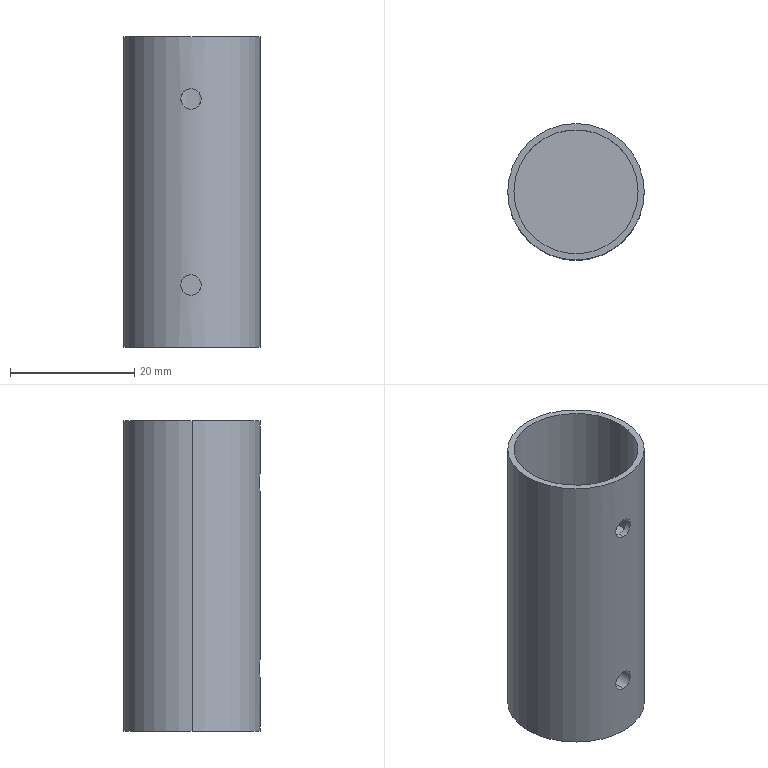Part | NX | 1 solid | 18 faces | box 22 x 22 x 50 mm | volume 7499 mm3 | plane 10 | cylinder 8 | commonest cylinder face diameters 3.3 x4 20 x2 22 x2
STEP:
#1=CARTESIAN_POINT('',(-0.1668,-10.999,38.35));
#2=VERTEX_POINT('',#1);
#3=CARTESIAN_POINT('',(-0.1668,-10.999,41.65));
#4=VERTEX_POINT('',#3);
#5=CARTESIAN_POINT('',(-0.1668,-10.999,38.35));
#6=CARTESIAN_POINT('',(-0.3506,-10.996,38.35));
#7=CARTESIAN_POINT('',(-0.5369,-10.988,38.382));
#8=CARTESIAN_POINT('',(-0.7102,-10.977,38.442));
#9=CARTESIAN_POINT('',(-0.8833,-10.966,38.502));
#10=CARTESIAN_POINT('',(-1.048,-10.951,38.593));
#11=CARTESIAN_POINT('',(-1.192,-10.935,38.707));
#12=CARTESIAN_POINT('',(-1.336,-10.919,38.822));
#13=CARTESIAN_POINT('',(-1.463,-10.903,38.963));
#14=CARTESIAN_POINT('',(-1.562,-10.889,39.119));
#15=CARTESIAN_POINT('',(-1.661,-10.874,39.275));
#16=CARTESIAN_POINT('',(-1.734,-10.863,39.452));
#17=CARTESIAN_POINT('',(-1.775,-10.856,39.633));
#18=CARTESIAN_POINT('',(-1.816,-10.849,39.812));
#19=CARTESIAN_POINT('',(-1.827,-10.847,40.001));
#20=CARTESIAN_POINT('',(-1.807,-10.851,40.184));
#21=CARTESIAN_POINT('',(-1.786,-10.854,40.365));
#22=CARTESIAN_POINT('',(-1.735,-10.863,40.545));
#23=CARTESIAN_POINT('',(-1.656,-10.875,40.71));
#24=CARTESIAN_POINT('',(-1.578,-10.887,40.875));
#25=CARTESIAN_POINT('',(-1.47,-10.902,41.028));
#26=CARTESIAN_POINT('',(-1.342,-10.918,41.158));
#27=CARTESIAN_POINT('',(-1.212,-10.934,41.29));
#28=CARTESIAN_POINT('',(-1.058,-10.95,41.401));
#29=CARTESIAN_POINT('',(-0.8922,-10.964,41.482));
#30=CARTESIAN_POINT('',(-0.7258,-10.977,41.563));
#31=CARTESIAN_POINT('',(-0.5427,-10.988,41.617));
#32=CARTESIAN_POINT('',(-0.3582,-10.994,41.639));
#33=CARTESIAN_POINT('',(-0.2948,-10.996,41.646));
#34=CARTESIAN_POINT('',(-0.2308,-10.998,41.65));
#35=CARTESIAN_POINT('',(-0.1668,-10.999,41.65));
#36=B_SPLINE_CURVE_WITH_KNOTS('',3,(#5,#6,#7,#8,#9,#10,#11,#12,#13,#14,#15,#16,#17,#18,#19,#20,#21,#22,#23,#24,#25,#26,#27,#28,#29,#30,#31,#32,#33,#34,#35),.UNSPECIFIED.,.F.,.F.,(4,3,3,3,3,3,3,3,3,3,4),(0.,0.1067,0.2134,0.3209,0.4288,0.5357,0.6415,0.7478,0.8555,0.9634,1.),.UNSPECIFIED.);
#37=EDGE_CURVE('',#2,#4,#36,.T.);
#38=ORIENTED_EDGE('',*,*,#37,.F.);
#39=CARTESIAN_POINT('',(-0.1668,-9.999,38.35));
#40=VERTEX_POINT('',#39);
#41=CARTESIAN_POINT('',(-0.1668,-8.66,38.35));
#42=DIRECTION('',(0.,1.,0.));
#43=VECTOR('',#42,1.);
#44=LINE('',#41,#43);
#45=EDGE_CURVE('',#2,#40,#44,.T.);
#46=ORIENTED_EDGE('',*,*,#45,.T.);
#47=CARTESIAN_POINT('',(-0.1668,-9.999,41.65));
#48=VERTEX_POINT('',#47);
#49=CARTESIAN_POINT('',(-0.1668,-9.999,41.65));
#50=CARTESIAN_POINT('',(-0.3505,-9.996,41.65));
#51=CARTESIAN_POINT('',(-0.5365,-9.987,41.618));
#52=CARTESIAN_POINT('',(-0.7096,-9.975,41.558));
#53=CARTESIAN_POINT('',(-0.8825,-9.962,41.498));
#54=CARTESIAN_POINT('',(-1.047,-9.946,41.407));
#55=CARTESIAN_POINT('',(-1.191,-9.929,41.294));
#56=CARTESIAN_POINT('',(-1.335,-9.912,41.18));
#57=CARTESIAN_POINT('',(-1.462,-9.893,41.039));
#58=CARTESIAN_POINT('',(-1.561,-9.877,40.883));
#59=CARTESIAN_POINT('',(-1.66,-9.862,40.726));
#60=CARTESIAN_POINT('',(-1.734,-9.849,40.55));
#61=CARTESIAN_POINT('',(-1.775,-9.841,40.368));
#62=CARTESIAN_POINT('',(-1.816,-9.834,40.189));
#63=CARTESIAN_POINT('',(-1.827,-9.832,40.));
#64=CARTESIAN_POINT('',(-1.807,-9.835,39.817));
#65=CARTESIAN_POINT('',(-1.787,-9.839,39.637));
#66=CARTESIAN_POINT('',(-1.735,-9.849,39.457));
#67=CARTESIAN_POINT('',(-1.658,-9.862,39.293));
#68=CARTESIAN_POINT('',(-1.58,-9.875,39.128));
#69=CARTESIAN_POINT('',(-1.473,-9.892,38.975));
#70=CARTESIAN_POINT('',(-1.345,-9.909,38.845));
#71=CARTESIAN_POINT('',(-1.216,-9.927,38.713));
#72=CARTESIAN_POINT('',(-1.062,-9.945,38.602));
#73=CARTESIAN_POINT('',(-0.8961,-9.96,38.52));
#74=CARTESIAN_POINT('',(-0.7298,-9.975,38.438));
#75=CARTESIAN_POINT('',(-0.5466,-9.987,38.384));
#76=CARTESIAN_POINT('',(-0.362,-9.993,38.362));
#77=CARTESIAN_POINT('',(-0.2973,-9.996,38.354));
#78=CARTESIAN_POINT('',(-0.232,-9.998,38.35));
#79=CARTESIAN_POINT('',(-0.1668,-9.999,38.35));
#80=B_SPLINE_CURVE_WITH_KNOTS('',3,(#49,#50,#51,#52,#53,#54,#55,#56,#57,#58,#59,#60,#61,#62,#63,#64,#65,#66,#67,#68,#69,#70,#71,#72,#73,#74,#75,#76,#77,#78,#79),.UNSPECIFIED.,.F.,.F.,(4,3,3,3,3,3,3,3,3,3,4),(0.,0.1066,0.2131,0.3206,0.4287,0.5354,0.6409,0.747,0.8546,0.9626,1.),.UNSPECIFIED.);
#81=EDGE_CURVE('',#48,#40,#80,.T.);
#82=ORIENTED_EDGE('',*,*,#81,.F.);
#83=CARTESIAN_POINT('',(-0.1668,-8.66,41.65));
#84=DIRECTION('',(0.,1.,0.));
#85=VECTOR('',#84,1.);
#86=LINE('',#83,#85);
#87=EDGE_CURVE('',#4,#48,#86,.T.);
#88=ORIENTED_EDGE('',*,*,#87,.F.);
#89=EDGE_LOOP('',(#38,#46,#82,#88));
#90=FACE_OUTER_BOUND('',#89,.T.);
#91=CARTESIAN_POINT('',(-0.1668,-8.66,40.));
#92=DIRECTION('',(0.,1.,0.));
#93=DIRECTION('',(0.,0.,1.));
#94=AXIS2_PLACEMENT_3D('',#91,#92,#93);
#95=CYLINDRICAL_SURFACE('',#94,1.65);
#96=ADVANCED_FACE('',(#90),#95,.F.);
#97=CARTESIAN_POINT('',(-0.1668,-10.999,8.35));
#98=VERTEX_POINT('',#97);
#99=CARTESIAN_POINT('',(-0.1668,-10.999,11.65));
#100=VERTEX_POINT('',#99);
#101=CARTESIAN_POINT('',(-0.1668,-10.999,8.35));
#102=CARTESIAN_POINT('',(-0.3506,-10.996,8.35));
#103=CARTESIAN_POINT('',(-0.5369,-10.988,8.382));
#104=CARTESIAN_POINT('',(-0.7102,-10.977,8.442));
#105=CARTESIAN_POINT('',(-0.8833,-10.966,8.502));
#106=CARTESIAN_POINT('',(-1.048,-10.951,8.593));
#107=CARTESIAN_POINT('',(-1.192,-10.935,8.707));
#108=CARTESIAN_POINT('',(-1.336,-10.919,8.822));
#109=CARTESIAN_POINT('',(-1.463,-10.903,8.963));
#110=CARTESIAN_POINT('',(-1.562,-10.889,9.119));
#111=CARTESIAN_POINT('',(-1.661,-10.874,9.275));
#112=CARTESIAN_POINT('',(-1.734,-10.863,9.452));
#113=CARTESIAN_POINT('',(-1.775,-10.856,9.633));
#114=CARTESIAN_POINT('',(-1.816,-10.849,9.812));
#115=CARTESIAN_POINT('',(-1.827,-10.847,10.001));
#116=CARTESIAN_POINT('',(-1.807,-10.851,10.184));
#117=CARTESIAN_POINT('',(-1.786,-10.854,10.365));
#118=CARTESIAN_POINT('',(-1.735,-10.863,10.545));
#119=CARTESIAN_POINT('',(-1.656,-10.875,10.71));
#120=CARTESIAN_POINT('',(-1.578,-10.887,10.875));
#121=CARTESIAN_POINT('',(-1.47,-10.902,11.028));
#122=CARTESIAN_POINT('',(-1.342,-10.918,11.158));
#123=CARTESIAN_POINT('',(-1.212,-10.934,11.29));
#124=CARTESIAN_POINT('',(-1.058,-10.95,11.401));
#125=CARTESIAN_POINT('',(-0.8922,-10.964,11.482));
#126=CARTESIAN_POINT('',(-0.7258,-10.977,11.563));
#127=CARTESIAN_POINT('',(-0.5427,-10.988,11.617));
#128=CARTESIAN_POINT('',(-0.3582,-10.994,11.639));
#129=CARTESIAN_POINT('',(-0.2948,-10.996,11.646));
#130=CARTESIAN_POINT('',(-0.2308,-10.998,11.65));
#131=CARTESIAN_POINT('',(-0.1668,-10.999,11.65));
#132=B_SPLINE_CURVE_WITH_KNOTS('',3,(#101,#102,#103,#104,#105,#106,#107,#108,#109,#110,#111,#112,#113,#114,#115,#116,#117,#118,#119,#120,#121,#122,#123,#124,#125,#126,#127,#128,#129,#130,#131),.UNSPECIFIED.,.F.,.F.,(4,3,3,3,3,3,3,3,3,3,4),(0.,0.1067,0.2134,0.3209,0.4288,0.5357,0.6415,0.7478,0.8555,0.9634,1.),.UNSPECIFIED.);
#133=EDGE_CURVE('',#98,#100,#132,.T.);
#134=ORIENTED_EDGE('',*,*,#133,.F.);
#135=CARTESIAN_POINT('',(-0.1668,-8.66,8.35));
#136=VERTEX_POINT('',#135);
#137=CARTESIAN_POINT('',(-0.1668,-8.66,8.35));
#138=DIRECTION('',(0.,1.,0.));
#139=VECTOR('',#138,1.);
#140=LINE('',#137,#139);
#141=EDGE_CURVE('',#98,#136,#140,.T.);
#142=ORIENTED_EDGE('',*,*,#141,.T.);
#143=CARTESIAN_POINT('',(-0.1668,-8.66,11.65));
#144=VERTEX_POINT('',#143);
#145=CARTESIAN_POINT('',(-0.1668,-8.66,10.));
#146=DIRECTION('',(0.,1.,0.));
#147=DIRECTION('',(0.,0.,1.));
#148=AXIS2_PLACEMENT_3D('',#145,#146,#147);
#149=CIRCLE('',#148,1.65);
#150=EDGE_CURVE('',#136,#144,#149,.T.);
#151=ORIENTED_EDGE('',*,*,#150,.T.);
#152=CARTESIAN_POINT('',(-0.1668,-8.66,11.65));
#153=DIRECTION('',(0.,1.,0.));
#154=VECTOR('',#153,1.);
#155=LINE('',#152,#154);
#156=EDGE_CURVE('',#100,#144,#155,.T.);
#157=ORIENTED_EDGE('',*,*,#156,.F.);
#158=EDGE_LOOP('',(#134,#142,#151,#157));
#159=FACE_OUTER_BOUND('',#158,.T.);
#160=CARTESIAN_POINT('',(-0.1668,-8.66,10.));
#161=DIRECTION('',(0.,1.,0.));
#162=DIRECTION('',(0.,0.,1.));
#163=AXIS2_PLACEMENT_3D('',#160,#161,#162);
#164=CYLINDRICAL_SURFACE('',#163,1.65);
#165=ADVANCED_FACE('',(#159),#164,.F.);
#166=ORIENTED_EDGE('',*,*,#81,.T.);
#167=CARTESIAN_POINT('',(-0.1668,-9.999,38.35));
#168=CARTESIAN_POINT('',(0.01615,-10.002,38.35));
#169=CARTESIAN_POINT('',(0.2018,-9.999,38.381));
#170=CARTESIAN_POINT('',(0.3745,-9.993,38.441));
#171=CARTESIAN_POINT('',(0.5473,-9.987,38.501));
#172=CARTESIAN_POINT('',(0.7119,-9.976,38.592));
#173=CARTESIAN_POINT('',(0.8552,-9.963,38.705));
#174=CARTESIAN_POINT('',(0.9996,-9.951,38.819));
#175=CARTESIAN_POINT('',(1.126,-9.937,38.959));
#176=CARTESIAN_POINT('',(1.225,-9.925,39.114));
#177=CARTESIAN_POINT('',(1.324,-9.912,39.27));
#178=CARTESIAN_POINT('',(1.398,-9.902,39.446));
#179=CARTESIAN_POINT('',(1.44,-9.896,39.626));
#180=CARTESIAN_POINT('',(1.482,-9.89,39.806));
#181=CARTESIAN_POINT('',(1.493,-9.888,39.995));
#182=CARTESIAN_POINT('',(1.473,-9.891,40.178));
#183=CARTESIAN_POINT('',(1.454,-9.894,40.36));
#184=CARTESIAN_POINT('',(1.403,-9.901,40.541));
#185=CARTESIAN_POINT('',(1.325,-9.912,40.706));
#186=CARTESIAN_POINT('',(1.246,-9.922,40.871));
#187=CARTESIAN_POINT('',(1.139,-9.936,41.026));
#188=CARTESIAN_POINT('',(1.01,-9.949,41.156));
#189=CARTESIAN_POINT('',(0.8808,-9.962,41.288));
#190=CARTESIAN_POINT('',(0.7267,-9.975,41.399));
#191=CARTESIAN_POINT('',(0.5606,-9.984,41.481));
#192=CARTESIAN_POINT('',(0.3946,-9.994,41.563));
#193=CARTESIAN_POINT('',(0.2121,-9.999,41.617));
#194=CARTESIAN_POINT('',(0.0283,-10.,41.638));
#195=CARTESIAN_POINT('',(-0.03641,-10.,41.646));
#196=CARTESIAN_POINT('',(-0.1017,-10.,41.65));
#197=CARTESIAN_POINT('',(-0.1668,-9.999,41.65));
#198=B_SPLINE_CURVE_WITH_KNOTS('',3,(#167,#168,#169,#170,#171,#172,#173,#174,#175,#176,#177,#178,#179,#180,#181,#182,#183,#184,#185,#186,#187,#188,#189,#190,#191,#192,#193,#194,#195,#196,#197),.UNSPECIFIED.,.F.,.F.,(4,3,3,3,3,3,3,3,3,3,4),(0.,0.1063,0.2126,0.3197,0.4275,0.5346,0.6408,0.7474,0.855,0.9626,1.),.UNSPECIFIED.);
#199=EDGE_CURVE('',#40,#48,#198,.T.);
#200=ORIENTED_EDGE('',*,*,#199,.T.);
#201=EDGE_LOOP('',(#166,#200));
#202=FACE_BOUND('',#201,.T.);
#203=CARTESIAN_POINT('',(-10.,0.,30.));
#204=VERTEX_POINT('',#203);
#205=CARTESIAN_POINT('',(10.,0.,30.));
#206=VERTEX_POINT('',#205);
#207=CARTESIAN_POINT('',(0.,0.,30.));
#208=DIRECTION('',(0.,0.,1.));
#209=DIRECTION('',(1.,0.,0.));
#210=AXIS2_PLACEMENT_3D('',#207,#208,#209);
#211=CIRCLE('',#210,10.);
#212=EDGE_CURVE('',#204,#206,#211,.T.);
#213=ORIENTED_EDGE('',*,*,#212,.F.);
#214=CARTESIAN_POINT('',(-10.,0.,50.));
#215=VERTEX_POINT('',#214);
#216=CARTESIAN_POINT('',(-10.,0.,30.));
#217=DIRECTION('',(0.,0.,1.));
#218=VECTOR('',#217,1.);
#219=LINE('',#216,#218);
#220=EDGE_CURVE('',#204,#215,#219,.T.);
#221=ORIENTED_EDGE('',*,*,#220,.T.);
#222=CARTESIAN_POINT('',(10.,0.,50.));
#223=VERTEX_POINT('',#222);
#224=CARTESIAN_POINT('',(0.,0.,50.));
#225=DIRECTION('',(0.,0.,1.));
#226=DIRECTION('',(1.,0.,0.));
#227=AXIS2_PLACEMENT_3D('',#224,#225,#226);
#228=CIRCLE('',#227,10.);
#229=EDGE_CURVE('',#215,#223,#228,.T.);
#230=ORIENTED_EDGE('',*,*,#229,.T.);
#231=CARTESIAN_POINT('',(10.,0.,30.));
#232=DIRECTION('',(0.,0.,1.));
#233=VECTOR('',#232,1.);
#234=LINE('',#231,#233);
#235=EDGE_CURVE('',#206,#223,#234,.T.);
#236=ORIENTED_EDGE('',*,*,#235,.F.);
#237=EDGE_LOOP('',(#213,#221,#230,#236));
#238=FACE_BOUND('',#237,.T.);
#239=CARTESIAN_POINT('',(0.,0.,30.));
#240=DIRECTION('',(0.,0.,1.));
#241=DIRECTION('',(1.,0.,0.));
#242=AXIS2_PLACEMENT_3D('',#239,#240,#241);
#243=CYLINDRICAL_SURFACE('',#242,10.);
#244=ADVANCED_FACE('',(#202,#238),#243,.F.);
#245=CARTESIAN_POINT('',(11.,0.,50.));
#246=VERTEX_POINT('',#245);
#247=CARTESIAN_POINT('',(-11.,0.,50.));
#248=VERTEX_POINT('',#247);
#249=CARTESIAN_POINT('',(0.,0.,50.));
#250=DIRECTION('',(0.,0.,1.));
#251=DIRECTION('',(1.,0.,0.));
#252=AXIS2_PLACEMENT_3D('',#249,#250,#251);
#253=CIRCLE('',#252,11.);
#254=EDGE_CURVE('',#246,#248,#253,.T.);
#255=ORIENTED_EDGE('',*,*,#254,.F.);
#256=CARTESIAN_POINT('',(11.,0.,0.));
#257=VERTEX_POINT('',#256);
#258=CARTESIAN_POINT('',(11.,0.,50.));
#259=DIRECTION('',(0.,0.,1.));
#260=VECTOR('',#259,1.);
#261=LINE('',#258,#260);
#262=EDGE_CURVE('',#257,#246,#261,.T.);
#263=ORIENTED_EDGE('',*,*,#262,.F.);
#264=CARTESIAN_POINT('',(-11.,0.,0.));
#265=VERTEX_POINT('',#264);
#266=CARTESIAN_POINT('',(0.,0.,0.));
#267=DIRECTION('',(0.,0.,1.));
#268=DIRECTION('',(1.,0.,0.));
#269=AXIS2_PLACEMENT_3D('',#266,#267,#268);
#270=CIRCLE('',#269,11.);
#271=EDGE_CURVE('',#257,#265,#270,.T.);
#272=ORIENTED_EDGE('',*,*,#271,.T.);
#273=CARTESIAN_POINT('',(-11.,0.,50.));
#274=DIRECTION('',(0.,0.,1.));
#275=VECTOR('',#274,1.);
#276=LINE('',#273,#275);
#277=EDGE_CURVE('',#265,#248,#276,.T.);
#278=ORIENTED_EDGE('',*,*,#277,.T.);
#279=EDGE_LOOP('',(#255,#263,#272,#278));
#280=FACE_OUTER_BOUND('',#279,.T.);
#281=CARTESIAN_POINT('',(0.,0.,50.));
#282=DIRECTION('',(0.,0.,-1.));
#283=DIRECTION('',(-1.,0.,0.));
#284=AXIS2_PLACEMENT_3D('',#281,#282,#283);
#285=CYLINDRICAL_SURFACE('',#284,11.);
#286=ADVANCED_FACE('',(#280),#285,.T.);
#287=ORIENTED_EDGE('',*,*,#262,.T.);
#288=CARTESIAN_POINT('',(0.,0.,50.));
#289=DIRECTION('',(0.,0.,1.));
#290=DIRECTION('',(1.,0.,0.));
#291=AXIS2_PLACEMENT_3D('',#288,#289,#290);
#292=CIRCLE('',#291,11.);
#293=EDGE_CURVE('',#248,#246,#292,.T.);
#294=ORIENTED_EDGE('',*,*,#293,.F.);
#295=ORIENTED_EDGE('',*,*,#277,.F.);
#296=CARTESIAN_POINT('',(0.,0.,0.));
#297=DIRECTION('',(0.,0.,1.));
#298=DIRECTION('',(1.,0.,0.));
#299=AXIS2_PLACEMENT_3D('',#296,#297,#298);
#300=CIRCLE('',#299,11.);
#301=EDGE_CURVE('',#265,#257,#300,.T.);
#302=ORIENTED_EDGE('',*,*,#301,.T.);
#303=EDGE_LOOP('',(#287,#294,#295,#302));
#304=FACE_BOUND('',#303,.T.);
#305=CARTESIAN_POINT('',(-0.1668,-10.999,41.65));
#306=CARTESIAN_POINT('',(0.01644,-11.002,41.65));
#307=CARTESIAN_POINT('',(0.2023,-11.,41.619));
#308=CARTESIAN_POINT('',(0.3754,-10.994,41.558));
#309=CARTESIAN_POINT('',(0.5484,-10.988,41.498));
#310=CARTESIAN_POINT('',(0.7133,-10.978,41.408));
#311=CARTESIAN_POINT('',(0.8567,-10.967,41.294));
#312=CARTESIAN_POINT('',(1.001,-10.955,41.18));
#313=CARTESIAN_POINT('',(1.128,-10.942,41.04));
#314=CARTESIAN_POINT('',(1.226,-10.931,40.884));
#315=CARTESIAN_POINT('',(1.325,-10.92,40.728));
#316=CARTESIAN_POINT('',(1.399,-10.911,40.552));
#317=CARTESIAN_POINT('',(1.441,-10.905,40.372));
#318=CARTESIAN_POINT('',(1.482,-10.9,40.192));
#319=CARTESIAN_POINT('',(1.493,-10.898,40.003));
#320=CARTESIAN_POINT('',(1.473,-10.901,39.819));
#321=CARTESIAN_POINT('',(1.453,-10.904,39.637));
#322=CARTESIAN_POINT('',(1.402,-10.911,39.456));
#323=CARTESIAN_POINT('',(1.323,-10.92,39.291));
#324=CARTESIAN_POINT('',(1.244,-10.93,39.126));
#325=CARTESIAN_POINT('',(1.136,-10.942,38.971));
#326=CARTESIAN_POINT('',(1.007,-10.954,38.841));
#327=CARTESIAN_POINT('',(0.8776,-10.966,38.709));
#328=CARTESIAN_POINT('',(0.7232,-10.977,38.598));
#329=CARTESIAN_POINT('',(0.557,-10.986,38.517));
#330=CARTESIAN_POINT('',(0.3909,-10.994,38.436));
#331=CARTESIAN_POINT('',(0.2083,-11.,38.383));
#332=CARTESIAN_POINT('',(0.02454,-11.,38.361));
#333=CARTESIAN_POINT('',(-0.03893,-11.,38.354));
#334=CARTESIAN_POINT('',(-0.1029,-11.,38.35));
#335=CARTESIAN_POINT('',(-0.1668,-10.999,38.35));
#336=B_SPLINE_CURVE_WITH_KNOTS('',3,(#305,#306,#307,#308,#309,#310,#311,#312,#313,#314,#315,#316,#317,#318,#319,#320,#321,#322,#323,#324,#325,#326,#327,#328,#329,#330,#331,#332,#333,#334,#335),.UNSPECIFIED.,.F.,.F.,(4,3,3,3,3,3,3,3,3,3,4),(0.,0.1065,0.213,0.3201,0.4279,0.535,0.6414,0.7482,0.8558,0.9633,1.),.UNSPECIFIED.);
#337=EDGE_CURVE('',#4,#2,#336,.T.);
#338=ORIENTED_EDGE('',*,*,#337,.T.);
#339=ORIENTED_EDGE('',*,*,#37,.T.);
#340=EDGE_LOOP('',(#338,#339));
#341=FACE_BOUND('',#340,.T.);
#342=CARTESIAN_POINT('',(-0.1668,-10.999,11.65));
#343=CARTESIAN_POINT('',(0.01644,-11.002,11.65));
#344=CARTESIAN_POINT('',(0.2023,-11.,11.619));
#345=CARTESIAN_POINT('',(0.3754,-10.994,11.558));
#346=CARTESIAN_POINT('',(0.5484,-10.988,11.498));
#347=CARTESIAN_POINT('',(0.7133,-10.978,11.408));
#348=CARTESIAN_POINT('',(0.8567,-10.967,11.294));
#349=CARTESIAN_POINT('',(1.001,-10.955,11.18));
#350=CARTESIAN_POINT('',(1.128,-10.942,11.04));
#351=CARTESIAN_POINT('',(1.226,-10.931,10.884));
#352=CARTESIAN_POINT('',(1.325,-10.92,10.728));
#353=CARTESIAN_POINT('',(1.399,-10.911,10.552));
#354=CARTESIAN_POINT('',(1.441,-10.905,10.372));
#355=CARTESIAN_POINT('',(1.482,-10.9,10.192));
#356=CARTESIAN_POINT('',(1.493,-10.898,10.003));
#357=CARTESIAN_POINT('',(1.473,-10.901,9.819));
#358=CARTESIAN_POINT('',(1.453,-10.904,9.637));
#359=CARTESIAN_POINT('',(1.402,-10.911,9.456));
#360=CARTESIAN_POINT('',(1.323,-10.92,9.291));
#361=CARTESIAN_POINT('',(1.244,-10.93,9.126));
#362=CARTESIAN_POINT('',(1.136,-10.942,8.971));
#363=CARTESIAN_POINT('',(1.007,-10.954,8.841));
#364=CARTESIAN_POINT('',(0.8776,-10.966,8.709));
#365=CARTESIAN_POINT('',(0.7232,-10.977,8.598));
#366=CARTESIAN_POINT('',(0.557,-10.986,8.517));
#367=CARTESIAN_POINT('',(0.3909,-10.994,8.436));
#368=CARTESIAN_POINT('',(0.2083,-11.,8.383));
#369=CARTESIAN_POINT('',(0.02454,-11.,8.361));
#370=CARTESIAN_POINT('',(-0.03893,-11.,8.354));
#371=CARTESIAN_POINT('',(-0.1029,-11.,8.35));
#372=CARTESIAN_POINT('',(-0.1668,-10.999,8.35));
#373=B_SPLINE_CURVE_WITH_KNOTS('',3,(#342,#343,#344,#345,#346,#347,#348,#349,#350,#351,#352,#353,#354,#355,#356,#357,#358,#359,#360,#361,#362,#363,#364,#365,#366,#367,#368,#369,#370,#371,#372),.UNSPECIFIED.,.F.,.F.,(4,3,3,3,3,3,3,3,3,3,4),(0.,0.1065,0.213,0.3201,0.4279,0.535,0.6414,0.7482,0.8558,0.9633,1.),.UNSPECIFIED.);
#374=EDGE_CURVE('',#100,#98,#373,.T.);
#375=ORIENTED_EDGE('',*,*,#374,.T.);
#376=ORIENTED_EDGE('',*,*,#133,.T.);
#377=EDGE_LOOP('',(#375,#376));
#378=FACE_BOUND('',#377,.T.);
#379=CARTESIAN_POINT('',(0.,0.,50.));
#380=DIRECTION('',(0.,0.,-1.));
#381=DIRECTION('',(-1.,0.,0.));
#382=AXIS2_PLACEMENT_3D('',#379,#380,#381);
#383=CYLINDRICAL_SURFACE('',#382,11.);
#384=ADVANCED_FACE('',(#304,#341,#378),#383,.T.);
#385=CARTESIAN_POINT('',(0.,0.,50.));
#386=DIRECTION('',(0.,0.,1.));
#387=DIRECTION('',(1.,0.,0.));
#388=AXIS2_PLACEMENT_3D('',#385,#386,#387);
#389=CIRCLE('',#388,10.);
#390=EDGE_CURVE('',#223,#215,#389,.T.);
#391=ORIENTED_EDGE('',*,*,#390,.F.);
#392=ORIENTED_EDGE('',*,*,#229,.F.);
#393=EDGE_LOOP('',(#391,#392));
#394=FACE_BOUND('',#393,.T.);
#395=ORIENTED_EDGE('',*,*,#293,.T.);
#396=ORIENTED_EDGE('',*,*,#254,.T.);
#397=EDGE_LOOP('',(#395,#396));
#398=FACE_BOUND('',#397,.T.);
#399=CARTESIAN_POINT('',(0.,0.,50.));
#400=DIRECTION('',(0.,0.,1.));
#401=DIRECTION('',(1.,0.,0.));
#402=AXIS2_PLACEMENT_3D('',#399,#400,#401);
#403=PLANE('',#402);
#404=ADVANCED_FACE('',(#394,#398),#403,.T.);
#405=CARTESIAN_POINT('',(-5.,-8.66,0.));
#406=VERTEX_POINT('',#405);
#407=CARTESIAN_POINT('',(-10.,0.,0.));
#408=VERTEX_POINT('',#407);
#409=CARTESIAN_POINT('',(-13.585,6.21,0.));
#410=DIRECTION('',(-0.5,0.866,0.));
#411=VECTOR('',#410,1.);
#412=LINE('',#409,#411);
#413=EDGE_CURVE('',#406,#408,#412,.T.);
#414=ORIENTED_EDGE('',*,*,#413,.F.);
#415=CARTESIAN_POINT('',(5.,-8.66,0.));
#416=VERTEX_POINT('',#415);
#417=CARTESIAN_POINT('',(-24.341,-8.66,0.));
#418=DIRECTION('',(-1.,0.,0.));
#419=VECTOR('',#418,1.);
#420=LINE('',#417,#419);
#421=EDGE_CURVE('',#416,#406,#420,.T.);
#422=ORIENTED_EDGE('',*,*,#421,.F.);
#423=CARTESIAN_POINT('',(10.,0.,0.));
#424=VERTEX_POINT('',#423);
#425=CARTESIAN_POINT('',(1.415,-14.87,0.));
#426=DIRECTION('',(-0.5,-0.866,0.));
#427=VECTOR('',#426,1.);
#428=LINE('',#425,#427);
#429=EDGE_CURVE('',#424,#416,#428,.T.);
#430=ORIENTED_EDGE('',*,*,#429,.F.);
#431=CARTESIAN_POINT('',(5.,8.66,0.));
#432=VERTEX_POINT('',#431);
#433=CARTESIAN_POINT('',(1.415,14.87,0.));
#434=DIRECTION('',(0.5,-0.866,0.));
#435=VECTOR('',#434,1.);
#436=LINE('',#433,#435);
#437=EDGE_CURVE('',#432,#424,#436,.T.);
#438=ORIENTED_EDGE('',*,*,#437,.F.);
#439=CARTESIAN_POINT('',(-5.,8.66,0.));
#440=VERTEX_POINT('',#439);
#441=CARTESIAN_POINT('',(-24.341,8.66,0.));
#442=DIRECTION('',(1.,0.,0.));
#443=VECTOR('',#442,1.);
#444=LINE('',#441,#443);
#445=EDGE_CURVE('',#440,#432,#444,.T.);
#446=ORIENTED_EDGE('',*,*,#445,.F.);
#447=CARTESIAN_POINT('',(-13.585,-6.21,0.));
#448=DIRECTION('',(0.5,0.866,0.));
#449=VECTOR('',#448,1.);
#450=LINE('',#447,#449);
#451=EDGE_CURVE('',#408,#440,#450,.T.);
#452=ORIENTED_EDGE('',*,*,#451,.F.);
#453=EDGE_LOOP('',(#414,#422,#430,#438,#446,#452));
#454=FACE_BOUND('',#453,.T.);
#455=ORIENTED_EDGE('',*,*,#301,.F.);
#456=ORIENTED_EDGE('',*,*,#271,.F.);
#457=EDGE_LOOP('',(#455,#456));
#458=FACE_BOUND('',#457,.T.);
#459=CARTESIAN_POINT('',(0.,0.,0.));
#460=DIRECTION('',(0.,0.,1.));
#461=DIRECTION('',(1.,0.,0.));
#462=AXIS2_PLACEMENT_3D('',#459,#460,#461);
#463=PLANE('',#462);
#464=ADVANCED_FACE('',(#454,#458),#463,.F.);
#465=ORIENTED_EDGE('',*,*,#220,.F.);
#466=CARTESIAN_POINT('',(0.,0.,30.));
#467=DIRECTION('',(0.,0.,1.));
#468=DIRECTION('',(1.,0.,0.));
#469=AXIS2_PLACEMENT_3D('',#466,#467,#468);
#470=CIRCLE('',#469,10.);
#471=EDGE_CURVE('',#206,#204,#470,.T.);
#472=ORIENTED_EDGE('',*,*,#471,.F.);
#473=ORIENTED_EDGE('',*,*,#235,.T.);
#474=ORIENTED_EDGE('',*,*,#390,.T.);
#475=EDGE_LOOP('',(#465,#472,#473,#474));
#476=FACE_OUTER_BOUND('',#475,.T.);
#477=CARTESIAN_POINT('',(0.,0.,30.));
#478=DIRECTION('',(0.,0.,1.));
#479=DIRECTION('',(1.,0.,0.));
#480=AXIS2_PLACEMENT_3D('',#477,#478,#479);
#481=CYLINDRICAL_SURFACE('',#480,10.);
#482=ADVANCED_FACE('',(#476),#481,.F.);
#483=ORIENTED_EDGE('',*,*,#471,.T.);
#484=ORIENTED_EDGE('',*,*,#212,.T.);
#485=EDGE_LOOP('',(#483,#484));
#486=FACE_OUTER_BOUND('',#485,.T.);
#487=CARTESIAN_POINT('',(0.,0.,30.));
#488=DIRECTION('',(0.,0.,1.));
#489=DIRECTION('',(1.,0.,0.));
#490=AXIS2_PLACEMENT_3D('',#487,#488,#489);
#491=PLANE('',#490);
#492=ADVANCED_FACE('',(#486),#491,.T.);
#493=CARTESIAN_POINT('',(-0.1668,-8.66,10.));
#494=DIRECTION('',(0.,1.,0.));
#495=DIRECTION('',(0.,0.,1.));
#496=AXIS2_PLACEMENT_3D('',#493,#494,#495);
#497=CIRCLE('',#496,1.65);
#498=EDGE_CURVE('',#144,#136,#497,.T.);
#499=ORIENTED_EDGE('',*,*,#498,.F.);
#500=ORIENTED_EDGE('',*,*,#150,.F.);
#501=EDGE_LOOP('',(#499,#500));
#502=FACE_BOUND('',#501,.T.);
#503=ORIENTED_EDGE('',*,*,#421,.T.);
#504=CARTESIAN_POINT('',(-5.,-8.66,20.));
#505=VERTEX_POINT('',#504);
#506=CARTESIAN_POINT('',(-5.,-8.66,20.));
#507=DIRECTION('',(0.,0.,-1.));
#508=VECTOR('',#507,1.);
#509=LINE('',#506,#508);
#510=EDGE_CURVE('',#505,#406,#509,.T.);
#511=ORIENTED_EDGE('',*,*,#510,.F.);
#512=CARTESIAN_POINT('',(5.,-8.66,20.));
#513=VERTEX_POINT('',#512);
#514=CARTESIAN_POINT('',(-24.341,-8.66,20.));
#515=DIRECTION('',(-1.,0.,0.));
#516=VECTOR('',#515,1.);
#517=LINE('',#514,#516);
#518=EDGE_CURVE('',#513,#505,#517,.T.);
#519=ORIENTED_EDGE('',*,*,#518,.F.);
#520=CARTESIAN_POINT('',(5.,-8.66,20.));
#521=DIRECTION('',(0.,0.,-1.));
#522=VECTOR('',#521,1.);
#523=LINE('',#520,#522);
#524=EDGE_CURVE('',#513,#416,#523,.T.);
#525=ORIENTED_EDGE('',*,*,#524,.T.);
#526=EDGE_LOOP('',(#503,#511,#519,#525));
#527=FACE_BOUND('',#526,.T.);
#528=CARTESIAN_POINT('',(-24.341,-8.66,20.));
#529=DIRECTION('',(0.,-1.,0.));
#530=DIRECTION('',(1.,0.,0.));
#531=AXIS2_PLACEMENT_3D('',#528,#529,#530);
#532=PLANE('',#531);
#533=ADVANCED_FACE('',(#502,#527),#532,.F.);
#534=ORIENTED_EDGE('',*,*,#429,.T.);
#535=ORIENTED_EDGE('',*,*,#524,.F.);
#536=CARTESIAN_POINT('',(10.,0.,20.));
#537=VERTEX_POINT('',#536);
#538=CARTESIAN_POINT('',(1.415,-14.87,20.));
#539=DIRECTION('',(-0.5,-0.866,0.));
#540=VECTOR('',#539,1.);
#541=LINE('',#538,#540);
#542=EDGE_CURVE('',#537,#513,#541,.T.);
#543=ORIENTED_EDGE('',*,*,#542,.F.);
#544=CARTESIAN_POINT('',(10.,0.,20.));
#545=DIRECTION('',(0.,0.,-1.));
#546=VECTOR('',#545,1.);
#547=LINE('',#544,#546);
#548=EDGE_CURVE('',#537,#424,#547,.T.);
#549=ORIENTED_EDGE('',*,*,#548,.T.);
#550=EDGE_LOOP('',(#534,#535,#543,#549));
#551=FACE_OUTER_BOUND('',#550,.T.);
#552=CARTESIAN_POINT('',(1.415,-14.87,20.));
#553=DIRECTION('',(0.866,-0.5,0.));
#554=DIRECTION('',(0.5,0.866,0.));
#555=AXIS2_PLACEMENT_3D('',#552,#553,#554);
#556=PLANE('',#555);
#557=ADVANCED_FACE('',(#551),#556,.F.);
#558=ORIENTED_EDGE('',*,*,#437,.T.);
#559=ORIENTED_EDGE('',*,*,#548,.F.);
#560=CARTESIAN_POINT('',(5.,8.66,20.));
#561=VERTEX_POINT('',#560);
#562=CARTESIAN_POINT('',(1.415,14.87,20.));
#563=DIRECTION('',(0.5,-0.866,0.));
#564=VECTOR('',#563,1.);
#565=LINE('',#562,#564);
#566=EDGE_CURVE('',#561,#537,#565,.T.);
#567=ORIENTED_EDGE('',*,*,#566,.F.);
#568=CARTESIAN_POINT('',(5.,8.66,20.));
#569=DIRECTION('',(0.,0.,-1.));
#570=VECTOR('',#569,1.);
#571=LINE('',#568,#570);
#572=EDGE_CURVE('',#561,#432,#571,.T.);
#573=ORIENTED_EDGE('',*,*,#572,.T.);
#574=EDGE_LOOP('',(#558,#559,#567,#573));
#575=FACE_OUTER_BOUND('',#574,.T.);
#576=CARTESIAN_POINT('',(1.415,14.87,20.));
#577=DIRECTION('',(0.866,0.5,0.));
#578=DIRECTION('',(-0.5,0.866,0.));
#579=AXIS2_PLACEMENT_3D('',#576,#577,#578);
#580=PLANE('',#579);
#581=ADVANCED_FACE('',(#575),#580,.F.);
#582=ORIENTED_EDGE('',*,*,#445,.T.);
#583=ORIENTED_EDGE('',*,*,#572,.F.);
#584=CARTESIAN_POINT('',(-5.,8.66,20.));
#585=VERTEX_POINT('',#584);
#586=CARTESIAN_POINT('',(-24.341,8.66,20.));
#587=DIRECTION('',(1.,0.,0.));
#588=VECTOR('',#587,1.);
#589=LINE('',#586,#588);
#590=EDGE_CURVE('',#585,#561,#589,.T.);
#591=ORIENTED_EDGE('',*,*,#590,.F.);
#592=CARTESIAN_POINT('',(-5.,8.66,20.));
#593=DIRECTION('',(0.,0.,-1.));
#594=VECTOR('',#593,1.);
#595=LINE('',#592,#594);
#596=EDGE_CURVE('',#585,#440,#595,.T.);
#597=ORIENTED_EDGE('',*,*,#596,.T.);
#598=EDGE_LOOP('',(#582,#583,#591,#597));
#599=FACE_OUTER_BOUND('',#598,.T.);
#600=CARTESIAN_POINT('',(-24.341,8.66,20.));
#601=DIRECTION('',(0.,1.,0.));
#602=DIRECTION('',(-1.,0.,0.));
#603=AXIS2_PLACEMENT_3D('',#600,#601,#602);
#604=PLANE('',#603);
#605=ADVANCED_FACE('',(#599),#604,.F.);
#606=ORIENTED_EDGE('',*,*,#451,.T.);
#607=ORIENTED_EDGE('',*,*,#596,.F.);
#608=CARTESIAN_POINT('',(-10.,0.,20.));
#609=VERTEX_POINT('',#608);
#610=CARTESIAN_POINT('',(-13.585,-6.21,20.));
#611=DIRECTION('',(0.5,0.866,0.));
#612=VECTOR('',#611,1.);
#613=LINE('',#610,#612);
#614=EDGE_CURVE('',#609,#585,#613,.T.);
#615=ORIENTED_EDGE('',*,*,#614,.F.);
#616=CARTESIAN_POINT('',(-10.,0.,20.));
#617=DIRECTION('',(0.,0.,-1.));
#618=VECTOR('',#617,1.);
#619=LINE('',#616,#618);
#620=EDGE_CURVE('',#609,#408,#619,.T.);
#621=ORIENTED_EDGE('',*,*,#620,.T.);
#622=EDGE_LOOP('',(#606,#607,#615,#621));
#623=FACE_OUTER_BOUND('',#622,.T.);
#624=CARTESIAN_POINT('',(-13.585,-6.21,20.));
#625=DIRECTION('',(-0.866,0.5,0.));
#626=DIRECTION('',(-0.5,-0.866,0.));
#627=AXIS2_PLACEMENT_3D('',#624,#625,#626);
#628=PLANE('',#627);
#629=ADVANCED_FACE('',(#623),#628,.F.);
#630=ORIENTED_EDGE('',*,*,#413,.T.);
#631=ORIENTED_EDGE('',*,*,#620,.F.);
#632=CARTESIAN_POINT('',(-13.585,6.21,20.));
#633=DIRECTION('',(-0.5,0.866,0.));
#634=VECTOR('',#633,1.);
#635=LINE('',#632,#634);
#636=EDGE_CURVE('',#505,#609,#635,.T.);
#637=ORIENTED_EDGE('',*,*,#636,.F.);
#638=ORIENTED_EDGE('',*,*,#510,.T.);
#639=EDGE_LOOP('',(#630,#631,#637,#638));
#640=FACE_OUTER_BOUND('',#639,.T.);
#641=CARTESIAN_POINT('',(-13.585,6.21,20.));
#642=DIRECTION('',(-0.866,-0.5,0.));
#643=DIRECTION('',(0.5,-0.866,0.));
#644=AXIS2_PLACEMENT_3D('',#641,#642,#643);
#645=PLANE('',#644);
#646=ADVANCED_FACE('',(#640),#645,.F.);
#647=ORIENTED_EDGE('',*,*,#518,.T.);
#648=ORIENTED_EDGE('',*,*,#636,.T.);
#649=ORIENTED_EDGE('',*,*,#614,.T.);
#650=ORIENTED_EDGE('',*,*,#590,.T.);
#651=ORIENTED_EDGE('',*,*,#566,.T.);
#652=ORIENTED_EDGE('',*,*,#542,.T.);
#653=EDGE_LOOP('',(#647,#648,#649,#650,#651,#652));
#654=FACE_OUTER_BOUND('',#653,.T.);
#655=CARTESIAN_POINT('',(-24.341,0.,20.));
#656=DIRECTION('',(0.,0.,-1.));
#657=DIRECTION('',(-1.,0.,0.));
#658=AXIS2_PLACEMENT_3D('',#655,#656,#657);
#659=PLANE('',#658);
#660=ADVANCED_FACE('',(#654),#659,.T.);
#661=ORIENTED_EDGE('',*,*,#141,.F.);
#662=ORIENTED_EDGE('',*,*,#374,.F.);
#663=ORIENTED_EDGE('',*,*,#156,.T.);
#664=ORIENTED_EDGE('',*,*,#498,.T.);
#665=EDGE_LOOP('',(#661,#662,#663,#664));
#666=FACE_OUTER_BOUND('',#665,.T.);
#667=CARTESIAN_POINT('',(-0.1668,-8.66,10.));
#668=DIRECTION('',(0.,1.,0.));
#669=DIRECTION('',(0.,0.,1.));
#670=AXIS2_PLACEMENT_3D('',#667,#668,#669);
#671=CYLINDRICAL_SURFACE('',#670,1.65);
#672=ADVANCED_FACE('',(#666),#671,.F.);
#673=ORIENTED_EDGE('',*,*,#45,.F.);
#674=ORIENTED_EDGE('',*,*,#337,.F.);
#675=ORIENTED_EDGE('',*,*,#87,.T.);
#676=ORIENTED_EDGE('',*,*,#199,.F.);
#677=EDGE_LOOP('',(#673,#674,#675,#676));
#678=FACE_OUTER_BOUND('',#677,.T.);
#679=CARTESIAN_POINT('',(-0.1668,-8.66,40.));
#680=DIRECTION('',(0.,1.,0.));
#681=DIRECTION('',(0.,0.,1.));
#682=AXIS2_PLACEMENT_3D('',#679,#680,#681);
#683=CYLINDRICAL_SURFACE('',#682,1.65);
#684=ADVANCED_FACE('',(#678),#683,.F.);
#685=CLOSED_SHELL('',(#96,#165,#244,#286,#384,#404,#464,#482,#492,#533,#557,#581,#605,#629,#646,#660,#672,#684));
#686=MANIFOLD_SOLID_BREP('',#685);
#687=(LENGTH_UNIT()NAMED_UNIT(*)SI_UNIT(.MILLI.,.METRE.));
#688=UNCERTAINTY_MEASURE_WITH_UNIT(LENGTH_MEASURE(0.0508),#687,'','');
#689=(NAMED_UNIT(*)PLANE_ANGLE_UNIT()SI_UNIT($,.RADIAN.));
#690=PLANE_ANGLE_MEASURE_WITH_UNIT(PLANE_ANGLE_MEASURE(0.01745),#689);
#691=DIMENSIONAL_EXPONENTS(0.,0.,0.,0.,0.,0.,0.);
#692=(CONVERSION_BASED_UNIT('DEGREE',#690)NAMED_UNIT(#691)PLANE_ANGLE_UNIT());
#693=(NAMED_UNIT(*)SI_UNIT($,.STERADIAN.)SOLID_ANGLE_UNIT());
#694=(GEOMETRIC_REPRESENTATION_CONTEXT(3)GLOBAL_UNCERTAINTY_ASSIGNED_CONTEXT((#688))GLOBAL_UNIT_ASSIGNED_CONTEXT((#687,#692,#693))REPRESENTATION_CONTEXT('',''));
#695=ADVANCED_BREP_SHAPE_REPRESENTATION('',(#686),#694);